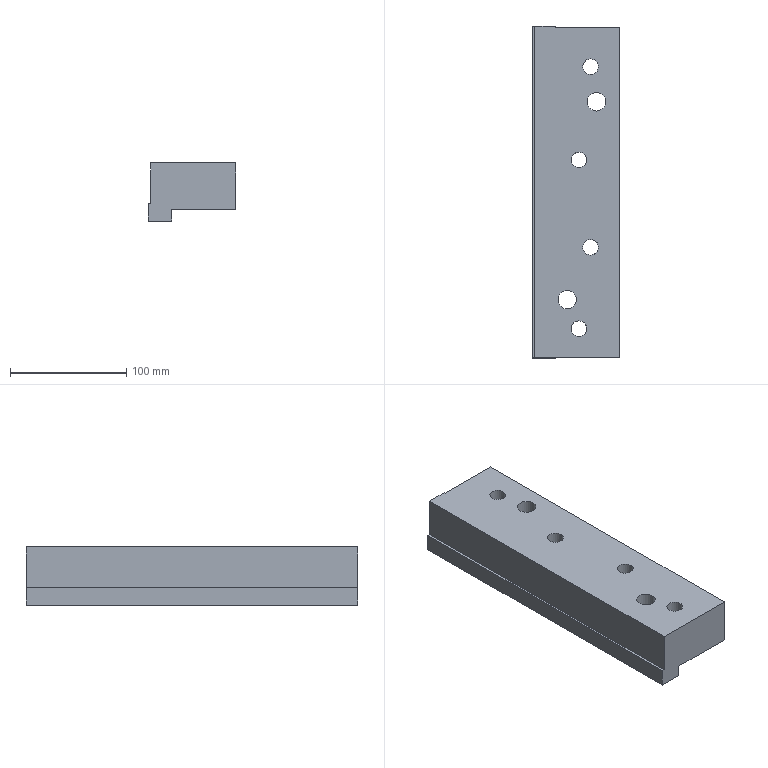Part | NX | features solid 2 | 1 solid | 25 faces | box 75 x 285 x 50 mm | volume 841532 mm3 | plane 15 | cylinder 10 | commonest cylinder face diameters 13.5 x4 19.5 x4 16 x2
STEP:
#1=CARTESIAN_POINT('',(1320.,-156.,43.));
#2=VERTEX_POINT('',#1);
#3=CARTESIAN_POINT('',(1320.,-156.,3.));
#4=VERTEX_POINT('',#3);
#5=CARTESIAN_POINT('',(1320.,-156.,-7.));
#6=DIRECTION('',(0.,0.,-1.));
#7=VECTOR('',#6,1000.);
#8=LINE('',#5,#7);
#9=EDGE_CURVE('',#2,#4,#8,.T.);
#10=ORIENTED_EDGE('',*,*,#9,.F.);
#11=CARTESIAN_POINT('',(1320.,-440.,43.));
#12=VERTEX_POINT('',#11);
#13=CARTESIAN_POINT('',(1320.,330.,43.));
#14=DIRECTION('',(0.,-1.,0.));
#15=VECTOR('',#14,1000.);
#16=LINE('',#13,#15);
#17=EDGE_CURVE('',#2,#12,#16,.T.);
#18=ORIENTED_EDGE('',*,*,#17,.T.);
#19=CARTESIAN_POINT('',(1320.,-440.,3.));
#20=VERTEX_POINT('',#19);
#21=CARTESIAN_POINT('',(1320.,-440.,-7.));
#22=DIRECTION('',(0.,0.,-1.));
#23=VECTOR('',#22,1000.);
#24=LINE('',#21,#23);
#25=EDGE_CURVE('',#20,#12,#24,.F.);
#26=ORIENTED_EDGE('',*,*,#25,.F.);
#27=CARTESIAN_POINT('',(1320.,330.,3.));
#28=DIRECTION('',(0.,-1.,0.));
#29=VECTOR('',#28,1000.);
#30=LINE('',#27,#29);
#31=EDGE_CURVE('',#4,#20,#30,.T.);
#32=ORIENTED_EDGE('',*,*,#31,.F.);
#33=EDGE_LOOP('',(#10,#18,#26,#32));
#34=FACE_BOUND('',#33,.T.);
#35=CARTESIAN_POINT('',(1320.,330.,-7.));
#36=DIRECTION('',(-1.,0.,0.));
#37=DIRECTION('',(0.,0.,1.));
#38=AXIS2_PLACEMENT_3D('',#35,#36,#37);
#39=PLANE('',#38);
#40=ADVANCED_FACE('',(#34),#39,.F.);
#41=CARTESIAN_POINT('',(1275.,-382.,43.));
#42=VERTEX_POINT('',#41);
#43=CARTESIAN_POINT('',(1275.,-390.,43.));
#44=DIRECTION('',(0.,0.,-1.));
#45=DIRECTION('',(0.,1.,0.));
#46=AXIS2_PLACEMENT_3D('',#43,#44,#45);
#47=CIRCLE('',#46,8.);
#48=EDGE_CURVE('',#42,#42,#47,.F.);
#49=ORIENTED_EDGE('',*,*,#48,.F.);
#50=EDGE_LOOP('',(#49));
#51=FACE_BOUND('',#50,.T.);
#52=CARTESIAN_POINT('',(1295.,-183.25,43.));
#53=VERTEX_POINT('',#52);
#54=CARTESIAN_POINT('',(1295.,-190.,43.));
#55=DIRECTION('',(0.,0.,-1.));
#56=DIRECTION('',(0.,1.,0.));
#57=AXIS2_PLACEMENT_3D('',#54,#55,#56);
#58=CIRCLE('',#57,6.75);
#59=EDGE_CURVE('',#53,#53,#58,.F.);
#60=ORIENTED_EDGE('',*,*,#59,.F.);
#61=EDGE_LOOP('',(#60));
#62=FACE_BOUND('',#61,.T.);
#63=CARTESIAN_POINT('',(1295.,-338.25,43.));
#64=VERTEX_POINT('',#63);
#65=CARTESIAN_POINT('',(1295.,-345.,43.));
#66=DIRECTION('',(0.,0.,-1.));
#67=DIRECTION('',(0.,1.,0.));
#68=AXIS2_PLACEMENT_3D('',#65,#66,#67);
#69=CIRCLE('',#68,6.75);
#70=EDGE_CURVE('',#64,#64,#69,.F.);
#71=ORIENTED_EDGE('',*,*,#70,.F.);
#72=EDGE_LOOP('',(#71));
#73=FACE_BOUND('',#72,.T.);
#74=CARTESIAN_POINT('',(1265.,-156.,43.));
#75=VERTEX_POINT('',#74);
#76=CARTESIAN_POINT('',(1319.,-156.,43.));
#77=DIRECTION('',(1.,0.,0.));
#78=VECTOR('',#77,1000.);
#79=LINE('',#76,#78);
#80=EDGE_CURVE('',#75,#2,#79,.T.);
#81=ORIENTED_EDGE('',*,*,#80,.F.);
#82=CARTESIAN_POINT('',(1265.,-155.,43.));
#83=VERTEX_POINT('',#82);
#84=CARTESIAN_POINT('',(1265.,-155.,43.));
#85=DIRECTION('',(0.,-1.,0.));
#86=VECTOR('',#85,1000.);
#87=LINE('',#84,#86);
#88=EDGE_CURVE('',#75,#83,#87,.F.);
#89=ORIENTED_EDGE('',*,*,#88,.T.);
#90=CARTESIAN_POINT('',(1247.,-155.,43.));
#91=VERTEX_POINT('',#90);
#92=CARTESIAN_POINT('',(1245.,-155.,43.));
#93=DIRECTION('',(1.,0.,0.));
#94=VECTOR('',#93,1000.);
#95=LINE('',#92,#94);
#96=EDGE_CURVE('',#91,#83,#95,.T.);
#97=ORIENTED_EDGE('',*,*,#96,.F.);
#98=CARTESIAN_POINT('',(1247.,-440.,43.));
#99=VERTEX_POINT('',#98);
#100=CARTESIAN_POINT('',(1247.,390.,43.));
#101=DIRECTION('',(0.,1.,0.));
#102=VECTOR('',#101,1000.);
#103=LINE('',#100,#102);
#104=EDGE_CURVE('',#91,#99,#103,.F.);
#105=ORIENTED_EDGE('',*,*,#104,.T.);
#106=CARTESIAN_POINT('',(1245.,-440.,43.));
#107=DIRECTION('',(-1.,0.,0.));
#108=VECTOR('',#107,1000.);
#109=LINE('',#106,#108);
#110=EDGE_CURVE('',#99,#12,#109,.F.);
#111=ORIENTED_EDGE('',*,*,#110,.T.);
#112=ORIENTED_EDGE('',*,*,#17,.F.);
#113=EDGE_LOOP('',(#81,#89,#97,#105,#111,#112));
#114=FACE_BOUND('',#113,.T.);
#115=CARTESIAN_POINT('',(1285.,-408.25,43.));
#116=VERTEX_POINT('',#115);
#117=CARTESIAN_POINT('',(1285.,-415.,43.));
#118=DIRECTION('',(0.,0.,-1.));
#119=DIRECTION('',(0.,1.,0.));
#120=AXIS2_PLACEMENT_3D('',#117,#118,#119);
#121=CIRCLE('',#120,6.75);
#122=EDGE_CURVE('',#116,#116,#121,.F.);
#123=ORIENTED_EDGE('',*,*,#122,.F.);
#124=EDGE_LOOP('',(#123));
#125=FACE_BOUND('',#124,.T.);
#126=CARTESIAN_POINT('',(1285.,-263.25,43.));
#127=VERTEX_POINT('',#126);
#128=CARTESIAN_POINT('',(1285.,-270.,43.));
#129=DIRECTION('',(0.,0.,-1.));
#130=DIRECTION('',(0.,1.,0.));
#131=AXIS2_PLACEMENT_3D('',#128,#129,#130);
#132=CIRCLE('',#131,6.75);
#133=EDGE_CURVE('',#127,#127,#132,.F.);
#134=ORIENTED_EDGE('',*,*,#133,.F.);
#135=EDGE_LOOP('',(#134));
#136=FACE_BOUND('',#135,.T.);
#137=CARTESIAN_POINT('',(1300.,-212.,43.));
#138=VERTEX_POINT('',#137);
#139=CARTESIAN_POINT('',(1300.,-220.,43.));
#140=DIRECTION('',(0.,0.,-1.));
#141=DIRECTION('',(0.,1.,0.));
#142=AXIS2_PLACEMENT_3D('',#139,#140,#141);
#143=CIRCLE('',#142,8.);
#144=EDGE_CURVE('',#138,#138,#143,.F.);
#145=ORIENTED_EDGE('',*,*,#144,.F.);
#146=EDGE_LOOP('',(#145));
#147=FACE_BOUND('',#146,.T.);
#148=CARTESIAN_POINT('',(1245.,390.,43.));
#149=DIRECTION('',(0.,0.,-1.));
#150=DIRECTION('',(0.,-1.,0.));
#151=AXIS2_PLACEMENT_3D('',#148,#149,#150);
#152=PLANE('',#151);
#153=ADVANCED_FACE('',(#51,#62,#73,#114,#125,#136,#147),#152,.F.);
#154=CARTESIAN_POINT('',(1265.,-156.,3.));
#155=VERTEX_POINT('',#154);
#156=CARTESIAN_POINT('',(1265.,-440.,3.));
#157=VERTEX_POINT('',#156);
#158=CARTESIAN_POINT('',(1265.,-155.,3.));
#159=DIRECTION('',(0.,-1.,0.));
#160=VECTOR('',#159,1000.);
#161=LINE('',#158,#160);
#162=EDGE_CURVE('',#155,#157,#161,.T.);
#163=ORIENTED_EDGE('',*,*,#162,.F.);
#164=CARTESIAN_POINT('',(1265.,-156.,3.));
#165=DIRECTION('',(1.,0.,0.));
#166=VECTOR('',#165,1000.);
#167=LINE('',#164,#166);
#168=EDGE_CURVE('',#155,#4,#167,.T.);
#169=ORIENTED_EDGE('',*,*,#168,.T.);
#170=ORIENTED_EDGE('',*,*,#31,.T.);
#171=CARTESIAN_POINT('',(1265.,-440.,3.));
#172=DIRECTION('',(-1.,0.,0.));
#173=VECTOR('',#172,1000.);
#174=LINE('',#171,#173);
#175=EDGE_CURVE('',#157,#20,#174,.F.);
#176=ORIENTED_EDGE('',*,*,#175,.F.);
#177=EDGE_LOOP('',(#163,#169,#170,#176));
#178=FACE_BOUND('',#177,.T.);
#179=CARTESIAN_POINT('',(1295.,-335.25,3.));
#180=VERTEX_POINT('',#179);
#181=CARTESIAN_POINT('',(1295.,-345.,3.));
#182=DIRECTION('',(0.,0.,-1.));
#183=DIRECTION('',(0.,1.,0.));
#184=AXIS2_PLACEMENT_3D('',#181,#182,#183);
#185=CIRCLE('',#184,9.75);
#186=EDGE_CURVE('',#180,#180,#185,.F.);
#187=ORIENTED_EDGE('',*,*,#186,.T.);
#188=EDGE_LOOP('',(#187));
#189=FACE_BOUND('',#188,.T.);
#190=CARTESIAN_POINT('',(1295.,-180.25,3.));
#191=VERTEX_POINT('',#190);
#192=CARTESIAN_POINT('',(1295.,-190.,3.));
#193=DIRECTION('',(0.,0.,-1.));
#194=DIRECTION('',(0.,1.,0.));
#195=AXIS2_PLACEMENT_3D('',#192,#193,#194);
#196=CIRCLE('',#195,9.75);
#197=EDGE_CURVE('',#191,#191,#196,.F.);
#198=ORIENTED_EDGE('',*,*,#197,.T.);
#199=EDGE_LOOP('',(#198));
#200=FACE_BOUND('',#199,.T.);
#201=CARTESIAN_POINT('',(1275.,-382.,3.));
#202=VERTEX_POINT('',#201);
#203=CARTESIAN_POINT('',(1275.,-390.,3.));
#204=DIRECTION('',(0.,0.,-1.));
#205=DIRECTION('',(0.,1.,0.));
#206=AXIS2_PLACEMENT_3D('',#203,#204,#205);
#207=CIRCLE('',#206,8.);
#208=EDGE_CURVE('',#202,#202,#207,.T.);
#209=ORIENTED_EDGE('',*,*,#208,.F.);
#210=EDGE_LOOP('',(#209));
#211=FACE_BOUND('',#210,.T.);
#212=CARTESIAN_POINT('',(1285.,-260.25,3.));
#213=VERTEX_POINT('',#212);
#214=CARTESIAN_POINT('',(1285.,-270.,3.));
#215=DIRECTION('',(0.,0.,-1.));
#216=DIRECTION('',(0.,1.,0.));
#217=AXIS2_PLACEMENT_3D('',#214,#215,#216);
#218=CIRCLE('',#217,9.75);
#219=EDGE_CURVE('',#213,#213,#218,.F.);
#220=ORIENTED_EDGE('',*,*,#219,.T.);
#221=EDGE_LOOP('',(#220));
#222=FACE_BOUND('',#221,.T.);
#223=CARTESIAN_POINT('',(1285.,-405.25,3.));
#224=VERTEX_POINT('',#223);
#225=CARTESIAN_POINT('',(1285.,-415.,3.));
#226=DIRECTION('',(0.,0.,-1.));
#227=DIRECTION('',(0.,1.,0.));
#228=AXIS2_PLACEMENT_3D('',#225,#226,#227);
#229=CIRCLE('',#228,9.75);
#230=EDGE_CURVE('',#224,#224,#229,.F.);
#231=ORIENTED_EDGE('',*,*,#230,.T.);
#232=EDGE_LOOP('',(#231));
#233=FACE_BOUND('',#232,.T.);
#234=CARTESIAN_POINT('',(1300.,-212.,3.));
#235=VERTEX_POINT('',#234);
#236=CARTESIAN_POINT('',(1300.,-220.,3.));
#237=DIRECTION('',(0.,0.,-1.));
#238=DIRECTION('',(0.,1.,0.));
#239=AXIS2_PLACEMENT_3D('',#236,#237,#238);
#240=CIRCLE('',#239,8.);
#241=EDGE_CURVE('',#235,#235,#240,.F.);
#242=ORIENTED_EDGE('',*,*,#241,.T.);
#243=EDGE_LOOP('',(#242));
#244=FACE_BOUND('',#243,.T.);
#245=CARTESIAN_POINT('',(1265.,-155.,3.));
#246=DIRECTION('',(0.,0.,-1.));
#247=DIRECTION('',(0.,-1.,0.));
#248=AXIS2_PLACEMENT_3D('',#245,#246,#247);
#249=PLANE('',#248);
#250=ADVANCED_FACE('',(#178,#189,#200,#211,#222,#233,#244),#249,.T.);
#251=ORIENTED_EDGE('',*,*,#175,.T.);
#252=ORIENTED_EDGE('',*,*,#25,.T.);
#253=ORIENTED_EDGE('',*,*,#110,.F.);
#254=CARTESIAN_POINT('',(1247.,-440.,8.));
#255=VERTEX_POINT('',#254);
#256=CARTESIAN_POINT('',(1247.,-440.,-7.));
#257=DIRECTION('',(0.,0.,1.));
#258=VECTOR('',#257,1000.);
#259=LINE('',#256,#258);
#260=EDGE_CURVE('',#99,#255,#259,.F.);
#261=ORIENTED_EDGE('',*,*,#260,.T.);
#262=CARTESIAN_POINT('',(1245.,-440.,8.));
#263=VERTEX_POINT('',#262);
#264=CARTESIAN_POINT('',(1245.,-440.,8.));
#265=DIRECTION('',(1.,0.,0.));
#266=VECTOR('',#265,1000.);
#267=LINE('',#264,#266);
#268=EDGE_CURVE('',#263,#255,#267,.T.);
#269=ORIENTED_EDGE('',*,*,#268,.F.);
#270=CARTESIAN_POINT('',(1245.,-440.,-7.));
#271=VERTEX_POINT('',#270);
#272=CARTESIAN_POINT('',(1245.,-440.,-7.));
#273=DIRECTION('',(0.,0.,-1.));
#274=VECTOR('',#273,1000.);
#275=LINE('',#272,#274);
#276=EDGE_CURVE('',#271,#263,#275,.F.);
#277=ORIENTED_EDGE('',*,*,#276,.F.);
#278=CARTESIAN_POINT('',(1265.,-440.,-7.));
#279=VERTEX_POINT('',#278);
#280=CARTESIAN_POINT('',(1245.,-440.,-7.));
#281=DIRECTION('',(1.,0.,0.));
#282=VECTOR('',#281,1000.);
#283=LINE('',#280,#282);
#284=EDGE_CURVE('',#271,#279,#283,.T.);
#285=ORIENTED_EDGE('',*,*,#284,.T.);
#286=CARTESIAN_POINT('',(1265.,-440.,-7.));
#287=DIRECTION('',(0.,0.,1.));
#288=VECTOR('',#287,1000.);
#289=LINE('',#286,#288);
#290=EDGE_CURVE('',#279,#157,#289,.T.);
#291=ORIENTED_EDGE('',*,*,#290,.T.);
#292=EDGE_LOOP('',(#251,#252,#253,#261,#269,#277,#285,#291));
#293=FACE_BOUND('',#292,.T.);
#294=CARTESIAN_POINT('',(1245.,-440.,-7.));
#295=DIRECTION('',(0.,-1.,0.));
#296=DIRECTION('',(0.,0.,1.));
#297=AXIS2_PLACEMENT_3D('',#294,#295,#296);
#298=PLANE('',#297);
#299=ADVANCED_FACE('',(#293),#298,.T.);
#300=ORIENTED_EDGE('',*,*,#96,.T.);
#301=CARTESIAN_POINT('',(1265.,-155.,-7.));
#302=VERTEX_POINT('',#301);
#303=CARTESIAN_POINT('',(1265.,-155.,-7.));
#304=DIRECTION('',(0.,0.,1.));
#305=VECTOR('',#304,1000.);
#306=LINE('',#303,#305);
#307=EDGE_CURVE('',#302,#83,#306,.T.);
#308=ORIENTED_EDGE('',*,*,#307,.F.);
#309=CARTESIAN_POINT('',(1245.,-155.,-7.));
#310=VERTEX_POINT('',#309);
#311=CARTESIAN_POINT('',(1245.,-155.,-7.));
#312=DIRECTION('',(1.,0.,0.));
#313=VECTOR('',#312,1000.);
#314=LINE('',#311,#313);
#315=EDGE_CURVE('',#302,#310,#314,.F.);
#316=ORIENTED_EDGE('',*,*,#315,.T.);
#317=CARTESIAN_POINT('',(1245.,-155.,8.));
#318=VERTEX_POINT('',#317);
#319=CARTESIAN_POINT('',(1245.,-155.,-7.));
#320=DIRECTION('',(0.,0.,-1.));
#321=VECTOR('',#320,1000.);
#322=LINE('',#319,#321);
#323=EDGE_CURVE('',#318,#310,#322,.T.);
#324=ORIENTED_EDGE('',*,*,#323,.F.);
#325=CARTESIAN_POINT('',(1247.,-155.,8.));
#326=VERTEX_POINT('',#325);
#327=CARTESIAN_POINT('',(1245.,-155.,8.));
#328=DIRECTION('',(-1.,0.,0.));
#329=VECTOR('',#328,1000.);
#330=LINE('',#327,#329);
#331=EDGE_CURVE('',#318,#326,#330,.F.);
#332=ORIENTED_EDGE('',*,*,#331,.T.);
#333=CARTESIAN_POINT('',(1247.,-155.,43.));
#334=DIRECTION('',(0.,0.,1.));
#335=VECTOR('',#334,1000.);
#336=LINE('',#333,#335);
#337=EDGE_CURVE('',#326,#91,#336,.T.);
#338=ORIENTED_EDGE('',*,*,#337,.T.);
#339=EDGE_LOOP('',(#300,#308,#316,#324,#332,#338));
#340=FACE_BOUND('',#339,.T.);
#341=CARTESIAN_POINT('',(1305.,-155.,-7.));
#342=DIRECTION('',(0.,1.,0.));
#343=DIRECTION('',(0.,0.,1.));
#344=AXIS2_PLACEMENT_3D('',#341,#342,#343);
#345=PLANE('',#344);
#346=ADVANCED_FACE('',(#340),#345,.T.);
#347=CARTESIAN_POINT('',(1285.,-424.75,18.));
#348=VERTEX_POINT('',#347);
#349=CARTESIAN_POINT('',(1285.,-415.,18.));
#350=DIRECTION('',(0.,0.,1.));
#351=DIRECTION('',(0.,-1.,0.));
#352=AXIS2_PLACEMENT_3D('',#349,#350,#351);
#353=CIRCLE('',#352,9.75);
#354=EDGE_CURVE('',#348,#348,#353,.T.);
#355=ORIENTED_EDGE('',*,*,#354,.T.);
#356=EDGE_LOOP('',(#355));
#357=FACE_BOUND('',#356,.T.);
#358=ORIENTED_EDGE('',*,*,#230,.F.);
#359=EDGE_LOOP('',(#358));
#360=FACE_BOUND('',#359,.T.);
#361=CARTESIAN_POINT('',(1285.,-415.,-82.));
#362=DIRECTION('',(0.,0.,1.));
#363=DIRECTION('',(1.,0.,0.));
#364=AXIS2_PLACEMENT_3D('',#361,#362,#363);
#365=CYLINDRICAL_SURFACE('',#364,9.75);
#366=ADVANCED_FACE('',(#357,#360),#365,.F.);
#367=CARTESIAN_POINT('',(1295.,-354.75,18.));
#368=VERTEX_POINT('',#367);
#369=CARTESIAN_POINT('',(1295.,-345.,18.));
#370=DIRECTION('',(0.,0.,1.));
#371=DIRECTION('',(0.,-1.,0.));
#372=AXIS2_PLACEMENT_3D('',#369,#370,#371);
#373=CIRCLE('',#372,9.75);
#374=EDGE_CURVE('',#368,#368,#373,.T.);
#375=ORIENTED_EDGE('',*,*,#374,.T.);
#376=EDGE_LOOP('',(#375));
#377=FACE_BOUND('',#376,.T.);
#378=ORIENTED_EDGE('',*,*,#186,.F.);
#379=EDGE_LOOP('',(#378));
#380=FACE_BOUND('',#379,.T.);
#381=CARTESIAN_POINT('',(1295.,-345.,-82.));
#382=DIRECTION('',(0.,0.,1.));
#383=DIRECTION('',(1.,0.,0.));
#384=AXIS2_PLACEMENT_3D('',#381,#382,#383);
#385=CYLINDRICAL_SURFACE('',#384,9.75);
#386=ADVANCED_FACE('',(#377,#380),#385,.F.);
#387=CARTESIAN_POINT('',(1285.,-279.75,18.));
#388=VERTEX_POINT('',#387);
#389=CARTESIAN_POINT('',(1285.,-270.,18.));
#390=DIRECTION('',(0.,0.,1.));
#391=DIRECTION('',(0.,-1.,0.));
#392=AXIS2_PLACEMENT_3D('',#389,#390,#391);
#393=CIRCLE('',#392,9.75);
#394=EDGE_CURVE('',#388,#388,#393,.T.);
#395=ORIENTED_EDGE('',*,*,#394,.T.);
#396=EDGE_LOOP('',(#395));
#397=FACE_BOUND('',#396,.T.);
#398=ORIENTED_EDGE('',*,*,#219,.F.);
#399=EDGE_LOOP('',(#398));
#400=FACE_BOUND('',#399,.T.);
#401=CARTESIAN_POINT('',(1285.,-270.,-82.));
#402=DIRECTION('',(0.,0.,1.));
#403=DIRECTION('',(1.,0.,0.));
#404=AXIS2_PLACEMENT_3D('',#401,#402,#403);
#405=CYLINDRICAL_SURFACE('',#404,9.75);
#406=ADVANCED_FACE('',(#397,#400),#405,.F.);
#407=CARTESIAN_POINT('',(1295.,-199.75,18.));
#408=VERTEX_POINT('',#407);
#409=CARTESIAN_POINT('',(1295.,-190.,18.));
#410=DIRECTION('',(0.,0.,1.));
#411=DIRECTION('',(0.,-1.,0.));
#412=AXIS2_PLACEMENT_3D('',#409,#410,#411);
#413=CIRCLE('',#412,9.75);
#414=EDGE_CURVE('',#408,#408,#413,.T.);
#415=ORIENTED_EDGE('',*,*,#414,.T.);
#416=EDGE_LOOP('',(#415));
#417=FACE_BOUND('',#416,.T.);
#418=ORIENTED_EDGE('',*,*,#197,.F.);
#419=EDGE_LOOP('',(#418));
#420=FACE_BOUND('',#419,.T.);
#421=CARTESIAN_POINT('',(1295.,-190.,-82.));
#422=DIRECTION('',(0.,0.,1.));
#423=DIRECTION('',(1.,0.,0.));
#424=AXIS2_PLACEMENT_3D('',#421,#422,#423);
#425=CYLINDRICAL_SURFACE('',#424,9.75);
#426=ADVANCED_FACE('',(#417,#420),#425,.F.);
#427=ORIENTED_EDGE('',*,*,#48,.T.);
#428=EDGE_LOOP('',(#427));
#429=FACE_BOUND('',#428,.T.);
#430=ORIENTED_EDGE('',*,*,#208,.T.);
#431=EDGE_LOOP('',(#430));
#432=FACE_BOUND('',#431,.T.);
#433=CARTESIAN_POINT('',(1275.,-390.,93.));
#434=DIRECTION('',(0.,0.,-1.));
#435=DIRECTION('',(-1.,0.,0.));
#436=AXIS2_PLACEMENT_3D('',#433,#434,#435);
#437=CYLINDRICAL_SURFACE('',#436,8.);
#438=ADVANCED_FACE('',(#429,#432),#437,.F.);
#439=ORIENTED_EDGE('',*,*,#315,.F.);
#440=CARTESIAN_POINT('',(1265.,330.,-7.));
#441=DIRECTION('',(0.,1.,0.));
#442=VECTOR('',#441,1000.);
#443=LINE('',#440,#442);
#444=EDGE_CURVE('',#302,#279,#443,.F.);
#445=ORIENTED_EDGE('',*,*,#444,.T.);
#446=ORIENTED_EDGE('',*,*,#284,.F.);
#447=CARTESIAN_POINT('',(1245.,330.,-7.));
#448=DIRECTION('',(0.,1.,0.));
#449=VECTOR('',#448,1000.);
#450=LINE('',#447,#449);
#451=EDGE_CURVE('',#310,#271,#450,.F.);
#452=ORIENTED_EDGE('',*,*,#451,.F.);
#453=EDGE_LOOP('',(#439,#445,#446,#452));
#454=FACE_BOUND('',#453,.T.);
#455=CARTESIAN_POINT('',(1245.,330.,-7.));
#456=DIRECTION('',(0.,0.,-1.));
#457=DIRECTION('',(0.,-1.,0.));
#458=AXIS2_PLACEMENT_3D('',#455,#456,#457);
#459=PLANE('',#458);
#460=ADVANCED_FACE('',(#454),#459,.T.);
#461=CARTESIAN_POINT('',(1245.,390.,8.));
#462=DIRECTION('',(0.,-1.,0.));
#463=VECTOR('',#462,1000.);
#464=LINE('',#461,#463);
#465=EDGE_CURVE('',#318,#263,#464,.T.);
#466=ORIENTED_EDGE('',*,*,#465,.F.);
#467=ORIENTED_EDGE('',*,*,#323,.T.);
#468=ORIENTED_EDGE('',*,*,#451,.T.);
#469=ORIENTED_EDGE('',*,*,#276,.T.);
#470=EDGE_LOOP('',(#466,#467,#468,#469));
#471=FACE_BOUND('',#470,.T.);
#472=CARTESIAN_POINT('',(1245.,390.,-7.));
#473=DIRECTION('',(-1.,0.,0.));
#474=DIRECTION('',(0.,0.,1.));
#475=AXIS2_PLACEMENT_3D('',#472,#473,#474);
#476=PLANE('',#475);
#477=ADVANCED_FACE('',(#471),#476,.T.);
#478=ORIENTED_EDGE('',*,*,#331,.F.);
#479=ORIENTED_EDGE('',*,*,#465,.T.);
#480=ORIENTED_EDGE('',*,*,#268,.T.);
#481=CARTESIAN_POINT('',(1247.,390.,8.));
#482=DIRECTION('',(0.,1.,0.));
#483=VECTOR('',#482,1000.);
#484=LINE('',#481,#483);
#485=EDGE_CURVE('',#326,#255,#484,.F.);
#486=ORIENTED_EDGE('',*,*,#485,.F.);
#487=EDGE_LOOP('',(#478,#479,#480,#486));
#488=FACE_BOUND('',#487,.T.);
#489=CARTESIAN_POINT('',(1245.,390.,8.));
#490=DIRECTION('',(0.,0.,1.));
#491=DIRECTION('',(0.,-1.,0.));
#492=AXIS2_PLACEMENT_3D('',#489,#490,#491);
#493=PLANE('',#492);
#494=ADVANCED_FACE('',(#488),#493,.T.);
#495=ORIENTED_EDGE('',*,*,#337,.F.);
#496=ORIENTED_EDGE('',*,*,#485,.T.);
#497=ORIENTED_EDGE('',*,*,#260,.F.);
#498=ORIENTED_EDGE('',*,*,#104,.F.);
#499=EDGE_LOOP('',(#495,#496,#497,#498));
#500=FACE_BOUND('',#499,.T.);
#501=CARTESIAN_POINT('',(1247.,390.,43.));
#502=DIRECTION('',(1.,0.,0.));
#503=DIRECTION('',(0.,0.,-1.));
#504=AXIS2_PLACEMENT_3D('',#501,#502,#503);
#505=PLANE('',#504);
#506=ADVANCED_FACE('',(#500),#505,.F.);
#507=CARTESIAN_POINT('',(1291.75,-415.,18.));
#508=VERTEX_POINT('',#507);
#509=CARTESIAN_POINT('',(1285.,-415.,18.));
#510=DIRECTION('',(0.,0.,1.));
#511=DIRECTION('',(1.,0.,0.));
#512=AXIS2_PLACEMENT_3D('',#509,#510,#511);
#513=CIRCLE('',#512,6.75);
#514=EDGE_CURVE('',#508,#508,#513,.T.);
#515=ORIENTED_EDGE('',*,*,#514,.F.);
#516=EDGE_LOOP('',(#515));
#517=FACE_BOUND('',#516,.T.);
#518=ORIENTED_EDGE('',*,*,#122,.T.);
#519=EDGE_LOOP('',(#518));
#520=FACE_BOUND('',#519,.T.);
#521=CARTESIAN_POINT('',(1285.,-415.,118.));
#522=DIRECTION('',(0.,0.,-1.));
#523=DIRECTION('',(-1.,0.,0.));
#524=AXIS2_PLACEMENT_3D('',#521,#522,#523);
#525=CYLINDRICAL_SURFACE('',#524,6.75);
#526=ADVANCED_FACE('',(#517,#520),#525,.F.);
#527=CARTESIAN_POINT('',(1301.75,-345.,18.));
#528=VERTEX_POINT('',#527);
#529=CARTESIAN_POINT('',(1295.,-345.,18.));
#530=DIRECTION('',(0.,0.,1.));
#531=DIRECTION('',(1.,0.,0.));
#532=AXIS2_PLACEMENT_3D('',#529,#530,#531);
#533=CIRCLE('',#532,6.75);
#534=EDGE_CURVE('',#528,#528,#533,.T.);
#535=ORIENTED_EDGE('',*,*,#534,.F.);
#536=EDGE_LOOP('',(#535));
#537=FACE_BOUND('',#536,.T.);
#538=ORIENTED_EDGE('',*,*,#70,.T.);
#539=EDGE_LOOP('',(#538));
#540=FACE_BOUND('',#539,.T.);
#541=CARTESIAN_POINT('',(1295.,-345.,118.));
#542=DIRECTION('',(0.,0.,-1.));
#543=DIRECTION('',(-1.,0.,0.));
#544=AXIS2_PLACEMENT_3D('',#541,#542,#543);
#545=CYLINDRICAL_SURFACE('',#544,6.75);
#546=ADVANCED_FACE('',(#537,#540),#545,.F.);
#547=CARTESIAN_POINT('',(1291.75,-270.,18.));
#548=VERTEX_POINT('',#547);
#549=CARTESIAN_POINT('',(1285.,-270.,18.));
#550=DIRECTION('',(0.,0.,1.));
#551=DIRECTION('',(1.,0.,0.));
#552=AXIS2_PLACEMENT_3D('',#549,#550,#551);
#553=CIRCLE('',#552,6.75);
#554=EDGE_CURVE('',#548,#548,#553,.T.);
#555=ORIENTED_EDGE('',*,*,#554,.F.);
#556=EDGE_LOOP('',(#555));
#557=FACE_BOUND('',#556,.T.);
#558=ORIENTED_EDGE('',*,*,#133,.T.);
#559=EDGE_LOOP('',(#558));
#560=FACE_BOUND('',#559,.T.);
#561=CARTESIAN_POINT('',(1285.,-270.,118.));
#562=DIRECTION('',(0.,0.,-1.));
#563=DIRECTION('',(-1.,0.,0.));
#564=AXIS2_PLACEMENT_3D('',#561,#562,#563);
#565=CYLINDRICAL_SURFACE('',#564,6.75);
#566=ADVANCED_FACE('',(#557,#560),#565,.F.);
#567=CARTESIAN_POINT('',(1301.75,-190.,18.));
#568=VERTEX_POINT('',#567);
#569=CARTESIAN_POINT('',(1295.,-190.,18.));
#570=DIRECTION('',(0.,0.,1.));
#571=DIRECTION('',(1.,0.,0.));
#572=AXIS2_PLACEMENT_3D('',#569,#570,#571);
#573=CIRCLE('',#572,6.75);
#574=EDGE_CURVE('',#568,#568,#573,.T.);
#575=ORIENTED_EDGE('',*,*,#574,.F.);
#576=EDGE_LOOP('',(#575));
#577=FACE_BOUND('',#576,.T.);
#578=ORIENTED_EDGE('',*,*,#59,.T.);
#579=EDGE_LOOP('',(#578));
#580=FACE_BOUND('',#579,.T.);
#581=CARTESIAN_POINT('',(1295.,-190.,118.));
#582=DIRECTION('',(0.,0.,-1.));
#583=DIRECTION('',(-1.,0.,0.));
#584=AXIS2_PLACEMENT_3D('',#581,#582,#583);
#585=CYLINDRICAL_SURFACE('',#584,6.75);
#586=ADVANCED_FACE('',(#577,#580),#585,.F.);
#587=ORIENTED_EDGE('',*,*,#514,.T.);
#588=EDGE_LOOP('',(#587));
#589=FACE_BOUND('',#588,.T.);
#590=ORIENTED_EDGE('',*,*,#354,.F.);
#591=EDGE_LOOP('',(#590));
#592=FACE_BOUND('',#591,.T.);
#593=CARTESIAN_POINT('',(1285.,-415.,18.));
#594=DIRECTION('',(0.,0.,1.));
#595=DIRECTION('',(1.,0.,0.));
#596=AXIS2_PLACEMENT_3D('',#593,#594,#595);
#597=PLANE('',#596);
#598=ADVANCED_FACE('',(#589,#592),#597,.F.);
#599=ORIENTED_EDGE('',*,*,#534,.T.);
#600=EDGE_LOOP('',(#599));
#601=FACE_BOUND('',#600,.T.);
#602=ORIENTED_EDGE('',*,*,#374,.F.);
#603=EDGE_LOOP('',(#602));
#604=FACE_BOUND('',#603,.T.);
#605=CARTESIAN_POINT('',(1295.,-345.,18.));
#606=DIRECTION('',(0.,0.,1.));
#607=DIRECTION('',(1.,0.,0.));
#608=AXIS2_PLACEMENT_3D('',#605,#606,#607);
#609=PLANE('',#608);
#610=ADVANCED_FACE('',(#601,#604),#609,.F.);
#611=ORIENTED_EDGE('',*,*,#554,.T.);
#612=EDGE_LOOP('',(#611));
#613=FACE_BOUND('',#612,.T.);
#614=ORIENTED_EDGE('',*,*,#394,.F.);
#615=EDGE_LOOP('',(#614));
#616=FACE_BOUND('',#615,.T.);
#617=CARTESIAN_POINT('',(1285.,-270.,18.));
#618=DIRECTION('',(0.,0.,1.));
#619=DIRECTION('',(1.,0.,0.));
#620=AXIS2_PLACEMENT_3D('',#617,#618,#619);
#621=PLANE('',#620);
#622=ADVANCED_FACE('',(#613,#616),#621,.F.);
#623=ORIENTED_EDGE('',*,*,#574,.T.);
#624=EDGE_LOOP('',(#623));
#625=FACE_BOUND('',#624,.T.);
#626=ORIENTED_EDGE('',*,*,#414,.F.);
#627=EDGE_LOOP('',(#626));
#628=FACE_BOUND('',#627,.T.);
#629=CARTESIAN_POINT('',(1295.,-190.,18.));
#630=DIRECTION('',(0.,0.,1.));
#631=DIRECTION('',(1.,0.,0.));
#632=AXIS2_PLACEMENT_3D('',#629,#630,#631);
#633=PLANE('',#632);
#634=ADVANCED_FACE('',(#625,#628),#633,.F.);
#635=ORIENTED_EDGE('',*,*,#162,.T.);
#636=ORIENTED_EDGE('',*,*,#290,.F.);
#637=ORIENTED_EDGE('',*,*,#444,.F.);
#638=ORIENTED_EDGE('',*,*,#307,.T.);
#639=ORIENTED_EDGE('',*,*,#88,.F.);
#640=CARTESIAN_POINT('',(1265.,-156.,-7.));
#641=DIRECTION('',(0.,0.,-1.));
#642=VECTOR('',#641,1000.);
#643=LINE('',#640,#642);
#644=EDGE_CURVE('',#155,#75,#643,.F.);
#645=ORIENTED_EDGE('',*,*,#644,.F.);
#646=EDGE_LOOP('',(#635,#636,#637,#638,#639,#645));
#647=FACE_BOUND('',#646,.T.);
#648=CARTESIAN_POINT('',(1265.,-155.,-7.));
#649=DIRECTION('',(-1.,0.,0.));
#650=DIRECTION('',(0.,0.,1.));
#651=AXIS2_PLACEMENT_3D('',#648,#649,#650);
#652=PLANE('',#651);
#653=ADVANCED_FACE('',(#647),#652,.F.);
#654=ORIENTED_EDGE('',*,*,#241,.F.);
#655=EDGE_LOOP('',(#654));
#656=FACE_BOUND('',#655,.T.);
#657=ORIENTED_EDGE('',*,*,#144,.T.);
#658=EDGE_LOOP('',(#657));
#659=FACE_BOUND('',#658,.T.);
#660=CARTESIAN_POINT('',(1300.,-220.,103.));
#661=DIRECTION('',(0.,0.,-1.));
#662=DIRECTION('',(-1.,0.,0.));
#663=AXIS2_PLACEMENT_3D('',#660,#661,#662);
#664=CYLINDRICAL_SURFACE('',#663,8.);
#665=ADVANCED_FACE('',(#656,#659),#664,.F.);
#666=ORIENTED_EDGE('',*,*,#644,.T.);
#667=ORIENTED_EDGE('',*,*,#80,.T.);
#668=ORIENTED_EDGE('',*,*,#9,.T.);
#669=ORIENTED_EDGE('',*,*,#168,.F.);
#670=EDGE_LOOP('',(#666,#667,#668,#669));
#671=FACE_BOUND('',#670,.T.);
#672=CARTESIAN_POINT('',(1319.,-156.,-7.));
#673=DIRECTION('',(0.,1.,0.));
#674=DIRECTION('',(0.,0.,1.));
#675=AXIS2_PLACEMENT_3D('',#672,#673,#674);
#676=PLANE('',#675);
#677=ADVANCED_FACE('',(#671),#676,.T.);
#678=CLOSED_SHELL('',(#40,#153,#250,#299,#346,#366,#386,#406,#426,#438,#460,#477,#494,#506,#526,#546,#566,#586,#598,#610,#622,#634,#653,#665,#677));
#679=MANIFOLD_SOLID_BREP('',#678);
#680=(LENGTH_UNIT()NAMED_UNIT(*)SI_UNIT(.MILLI.,.METRE.));
#681=UNCERTAINTY_MEASURE_WITH_UNIT(LENGTH_MEASURE(0.00001),#680,'','');
#682=(NAMED_UNIT(*)PLANE_ANGLE_UNIT()SI_UNIT($,.RADIAN.));
#683=(NAMED_UNIT(*)SI_UNIT($,.STERADIAN.)SOLID_ANGLE_UNIT());
#684=(GEOMETRIC_REPRESENTATION_CONTEXT(3)GLOBAL_UNCERTAINTY_ASSIGNED_CONTEXT((#681))GLOBAL_UNIT_ASSIGNED_CONTEXT((#680,#682,#683))REPRESENTATION_CONTEXT('',''));
#685=ADVANCED_BREP_SHAPE_REPRESENTATION('',(#679),#684);